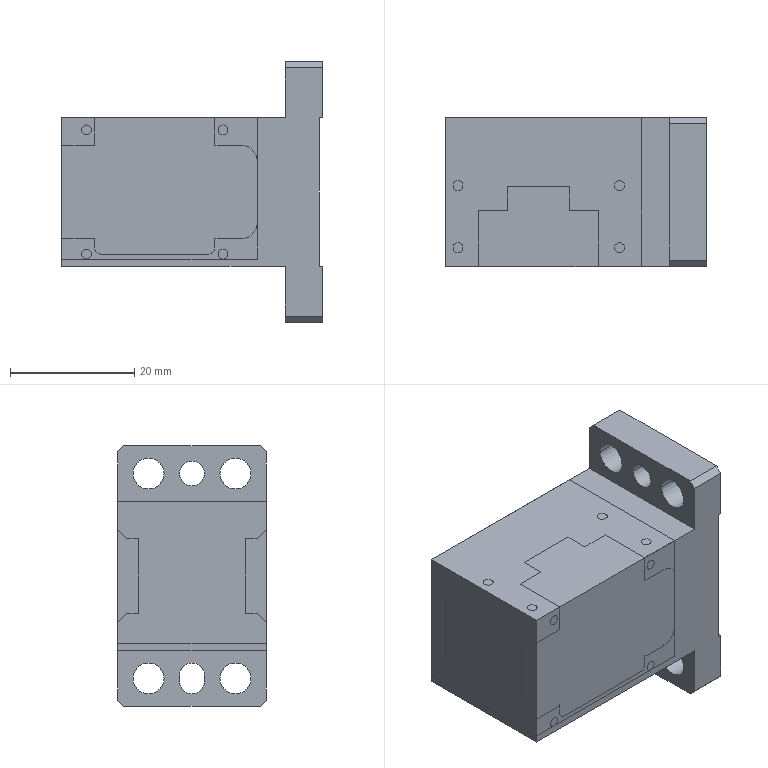NC program | NX | posted with a generic post | part box 42 x 24 x 42 mm
Lines 1 to 18 of 4089:
N10 G17 G21 G94 G90
(FLOOR_WALL , TOOL : D63)
N12 T01 M6
N14 G54
N16 G17 G0 G90 X-57.5 Y0. B0. C0. S2000 M3
N18 G43 Z30. H1
N20 Z3.
N22 G94 G1 Z0. F1200.
N24 X-54.5
N26 X54.5
N28 X57.5
N30 Z3.
N32 G0 Z30.
N34 M5